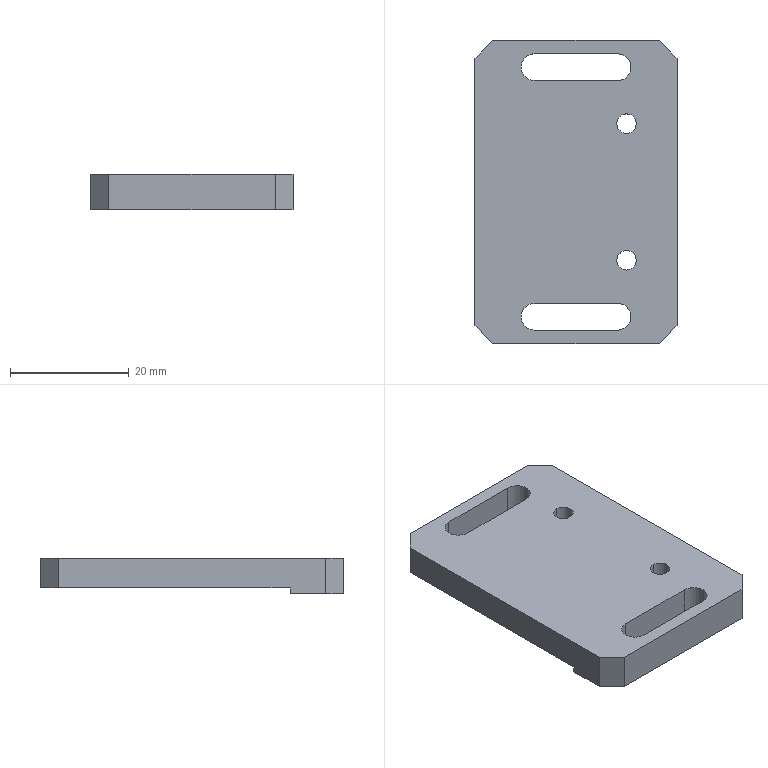Part | STEP file | 11-FG-SZ00711 | 1 solid | 26 faces | box 34 x 51 x 6 mm | volume 7924 mm3 | plane 16 | cylinder 10 | commonest cylinder face diameters 4.5 x6 3.3 x4
STEP:
#1=CARTESIAN_POINT('',(-9.25,21.,6.));
#2=VERTEX_POINT('',#1);
#3=CARTESIAN_POINT('',(-7.,23.25,6.));
#4=VERTEX_POINT('',#3);
#5=CARTESIAN_POINT('',(-7.,21.,6.));
#6=DIRECTION('',(0.,0.,-1.));
#7=DIRECTION('',(1.,0.,0.));
#8=AXIS2_PLACEMENT_3D('',#5,#6,#7);
#9=CIRCLE('',#8,2.25);
#10=EDGE_CURVE('',#2,#4,#9,.T.);
#11=ORIENTED_EDGE('',*,*,#10,.F.);
#12=CARTESIAN_POINT('',(-9.25,21.,1.));
#13=VERTEX_POINT('',#12);
#14=CARTESIAN_POINT('',(-9.25,21.,6.));
#15=DIRECTION('',(0.,0.,-1.));
#16=VECTOR('',#15,1000.);
#17=LINE('',#14,#16);
#18=EDGE_CURVE('',#2,#13,#17,.T.);
#19=ORIENTED_EDGE('',*,*,#18,.T.);
#20=CARTESIAN_POINT('',(-7.,23.25,1.));
#21=VERTEX_POINT('',#20);
#22=CARTESIAN_POINT('',(-7.,21.,1.));
#23=DIRECTION('',(0.,0.,1.));
#24=DIRECTION('',(0.,-1.,0.));
#25=AXIS2_PLACEMENT_3D('',#22,#23,#24);
#26=CIRCLE('',#25,2.25);
#27=EDGE_CURVE('',#21,#13,#26,.T.);
#28=ORIENTED_EDGE('',*,*,#27,.F.);
#29=CARTESIAN_POINT('',(-7.,23.25,6.));
#30=DIRECTION('',(0.,0.,-1.));
#31=VECTOR('',#30,1000.);
#32=LINE('',#29,#31);
#33=EDGE_CURVE('',#4,#21,#32,.T.);
#34=ORIENTED_EDGE('',*,*,#33,.F.);
#35=EDGE_LOOP('',(#11,#19,#28,#34));
#36=FACE_OUTER_BOUND('',#35,.T.);
#37=CARTESIAN_POINT('',(-7.,21.,6.));
#38=DIRECTION('',(0.,0.,-1.));
#39=DIRECTION('',(-1.,0.,0.));
#40=AXIS2_PLACEMENT_3D('',#37,#38,#39);
#41=CYLINDRICAL_SURFACE('',#40,2.25);
#42=ADVANCED_FACE('',(#36),#41,.F.);
#43=CARTESIAN_POINT('',(-9.25,-21.,6.));
#44=VERTEX_POINT('',#43);
#45=CARTESIAN_POINT('',(-7.,-18.75,6.));
#46=VERTEX_POINT('',#45);
#47=CARTESIAN_POINT('',(-7.,-21.,6.));
#48=DIRECTION('',(0.,0.,-1.));
#49=DIRECTION('',(-1.,0.,0.));
#50=AXIS2_PLACEMENT_3D('',#47,#48,#49);
#51=CIRCLE('',#50,2.25);
#52=EDGE_CURVE('',#44,#46,#51,.T.);
#53=ORIENTED_EDGE('',*,*,#52,.F.);
#54=CARTESIAN_POINT('',(-9.25,-21.,0.));
#55=VERTEX_POINT('',#54);
#56=CARTESIAN_POINT('',(-9.25,-21.,6.));
#57=DIRECTION('',(0.,0.,-1.));
#58=VECTOR('',#57,1000.);
#59=LINE('',#56,#58);
#60=EDGE_CURVE('',#44,#55,#59,.T.);
#61=ORIENTED_EDGE('',*,*,#60,.T.);
#62=CARTESIAN_POINT('',(-7.,-18.75,0.));
#63=VERTEX_POINT('',#62);
#64=CARTESIAN_POINT('',(-7.,-21.,0.));
#65=DIRECTION('',(0.,0.,-1.));
#66=DIRECTION('',(-1.,0.,0.));
#67=AXIS2_PLACEMENT_3D('',#64,#65,#66);
#68=CIRCLE('',#67,2.25);
#69=EDGE_CURVE('',#55,#63,#68,.T.);
#70=ORIENTED_EDGE('',*,*,#69,.T.);
#71=CARTESIAN_POINT('',(-7.,-18.75,6.));
#72=DIRECTION('',(0.,0.,-1.));
#73=VECTOR('',#72,1000.);
#74=LINE('',#71,#73);
#75=EDGE_CURVE('',#46,#63,#74,.T.);
#76=ORIENTED_EDGE('',*,*,#75,.F.);
#77=EDGE_LOOP('',(#53,#61,#70,#76));
#78=FACE_OUTER_BOUND('',#77,.T.);
#79=CARTESIAN_POINT('',(-7.,-21.,6.));
#80=DIRECTION('',(0.,0.,-1.));
#81=DIRECTION('',(-1.,0.,0.));
#82=AXIS2_PLACEMENT_3D('',#79,#80,#81);
#83=CYLINDRICAL_SURFACE('',#82,2.25);
#84=ADVANCED_FACE('',(#78),#83,.F.);
#85=CARTESIAN_POINT('',(8.5,-9.85,6.));
#86=VERTEX_POINT('',#85);
#87=CARTESIAN_POINT('',(8.5,-13.15,6.));
#88=VERTEX_POINT('',#87);
#89=CARTESIAN_POINT('',(8.5,-11.5,6.));
#90=DIRECTION('',(0.,0.,1.));
#91=DIRECTION('',(1.,0.,0.));
#92=AXIS2_PLACEMENT_3D('',#89,#90,#91);
#93=CIRCLE('',#92,1.65);
#94=EDGE_CURVE('',#86,#88,#93,.T.);
#95=ORIENTED_EDGE('',*,*,#94,.T.);
#96=CARTESIAN_POINT('',(8.5,-13.15,1.));
#97=VERTEX_POINT('',#96);
#98=CARTESIAN_POINT('',(8.5,-13.15,1.));
#99=DIRECTION('',(0.,0.,-1.));
#100=VECTOR('',#99,1000.);
#101=LINE('',#98,#100);
#102=EDGE_CURVE('',#88,#97,#101,.T.);
#103=ORIENTED_EDGE('',*,*,#102,.T.);
#104=CARTESIAN_POINT('',(8.5,-9.85,1.));
#105=VERTEX_POINT('',#104);
#106=CARTESIAN_POINT('',(8.5,-11.5,1.));
#107=DIRECTION('',(0.,0.,-1.));
#108=DIRECTION('',(0.,1.,0.));
#109=AXIS2_PLACEMENT_3D('',#106,#107,#108);
#110=CIRCLE('',#109,1.65);
#111=EDGE_CURVE('',#97,#105,#110,.T.);
#112=ORIENTED_EDGE('',*,*,#111,.T.);
#113=CARTESIAN_POINT('',(8.5,-9.85,1.));
#114=DIRECTION('',(0.,0.,-1.));
#115=VECTOR('',#114,1000.);
#116=LINE('',#113,#115);
#117=EDGE_CURVE('',#86,#105,#116,.T.);
#118=ORIENTED_EDGE('',*,*,#117,.F.);
#119=EDGE_LOOP('',(#95,#103,#112,#118));
#120=FACE_OUTER_BOUND('',#119,.T.);
#121=CARTESIAN_POINT('',(8.5,-11.5,1.));
#122=DIRECTION('',(0.,0.,-1.));
#123=DIRECTION('',(0.,1.,0.));
#124=AXIS2_PLACEMENT_3D('',#121,#122,#123);
#125=CYLINDRICAL_SURFACE('',#124,1.65);
#126=ADVANCED_FACE('',(#120),#125,.F.);
#127=CARTESIAN_POINT('',(8.5,13.15,6.));
#128=VERTEX_POINT('',#127);
#129=CARTESIAN_POINT('',(8.5,9.85,6.));
#130=VERTEX_POINT('',#129);
#131=CARTESIAN_POINT('',(8.5,11.5,6.));
#132=DIRECTION('',(0.,0.,1.));
#133=DIRECTION('',(1.,0.,0.));
#134=AXIS2_PLACEMENT_3D('',#131,#132,#133);
#135=CIRCLE('',#134,1.65);
#136=EDGE_CURVE('',#128,#130,#135,.T.);
#137=ORIENTED_EDGE('',*,*,#136,.T.);
#138=CARTESIAN_POINT('',(8.5,9.85,1.));
#139=VERTEX_POINT('',#138);
#140=CARTESIAN_POINT('',(8.5,9.85,1.));
#141=DIRECTION('',(0.,0.,-1.));
#142=VECTOR('',#141,1000.);
#143=LINE('',#140,#142);
#144=EDGE_CURVE('',#130,#139,#143,.T.);
#145=ORIENTED_EDGE('',*,*,#144,.T.);
#146=CARTESIAN_POINT('',(8.5,13.15,1.));
#147=VERTEX_POINT('',#146);
#148=CARTESIAN_POINT('',(8.5,11.5,1.));
#149=DIRECTION('',(0.,0.,-1.));
#150=DIRECTION('',(0.,1.,0.));
#151=AXIS2_PLACEMENT_3D('',#148,#149,#150);
#152=CIRCLE('',#151,1.65);
#153=EDGE_CURVE('',#139,#147,#152,.T.);
#154=ORIENTED_EDGE('',*,*,#153,.T.);
#155=CARTESIAN_POINT('',(8.5,13.15,1.));
#156=DIRECTION('',(0.,0.,-1.));
#157=VECTOR('',#156,1000.);
#158=LINE('',#155,#157);
#159=EDGE_CURVE('',#128,#147,#158,.T.);
#160=ORIENTED_EDGE('',*,*,#159,.F.);
#161=EDGE_LOOP('',(#137,#145,#154,#160));
#162=FACE_OUTER_BOUND('',#161,.T.);
#163=CARTESIAN_POINT('',(8.5,11.5,1.));
#164=DIRECTION('',(0.,0.,-1.));
#165=DIRECTION('',(0.,1.,0.));
#166=AXIS2_PLACEMENT_3D('',#163,#164,#165);
#167=CYLINDRICAL_SURFACE('',#166,1.65);
#168=ADVANCED_FACE('',(#162),#167,.F.);
#169=CARTESIAN_POINT('',(17.,22.5,1.));
#170=VERTEX_POINT('',#169);
#171=CARTESIAN_POINT('',(17.,-16.5,1.));
#172=VERTEX_POINT('',#171);
#173=CARTESIAN_POINT('',(17.,25.5,1.));
#174=DIRECTION('',(0.,-1.,0.));
#175=VECTOR('',#174,1000.);
#176=LINE('',#173,#175);
#177=EDGE_CURVE('',#170,#172,#176,.T.);
#178=ORIENTED_EDGE('',*,*,#177,.F.);
#179=CARTESIAN_POINT('',(17.,22.5,6.));
#180=VERTEX_POINT('',#179);
#181=CARTESIAN_POINT('',(17.,22.5,6.));
#182=DIRECTION('',(0.,0.,1.));
#183=VECTOR('',#182,1000.);
#184=LINE('',#181,#183);
#185=EDGE_CURVE('',#170,#180,#184,.T.);
#186=ORIENTED_EDGE('',*,*,#185,.T.);
#187=CARTESIAN_POINT('',(17.,-22.5,6.));
#188=VERTEX_POINT('',#187);
#189=CARTESIAN_POINT('',(17.,25.5,6.));
#190=DIRECTION('',(0.,1.,0.));
#191=VECTOR('',#190,1000.);
#192=LINE('',#189,#191);
#193=EDGE_CURVE('',#188,#180,#192,.T.);
#194=ORIENTED_EDGE('',*,*,#193,.F.);
#195=CARTESIAN_POINT('',(17.,-22.5,0.));
#196=VERTEX_POINT('',#195);
#197=CARTESIAN_POINT('',(17.,-22.5,6.));
#198=DIRECTION('',(0.,0.,-1.));
#199=VECTOR('',#198,1000.);
#200=LINE('',#197,#199);
#201=EDGE_CURVE('',#188,#196,#200,.T.);
#202=ORIENTED_EDGE('',*,*,#201,.T.);
#203=CARTESIAN_POINT('',(17.,-16.5,0.));
#204=VERTEX_POINT('',#203);
#205=CARTESIAN_POINT('',(17.,25.5,0.));
#206=DIRECTION('',(0.,1.,0.));
#207=VECTOR('',#206,1000.);
#208=LINE('',#205,#207);
#209=EDGE_CURVE('',#196,#204,#208,.T.);
#210=ORIENTED_EDGE('',*,*,#209,.T.);
#211=CARTESIAN_POINT('',(17.,-16.5,0.));
#212=DIRECTION('',(0.,0.,-1.));
#213=VECTOR('',#212,1000.);
#214=LINE('',#211,#213);
#215=EDGE_CURVE('',#172,#204,#214,.T.);
#216=ORIENTED_EDGE('',*,*,#215,.F.);
#217=EDGE_LOOP('',(#178,#186,#194,#202,#210,#216));
#218=FACE_OUTER_BOUND('',#217,.T.);
#219=CARTESIAN_POINT('',(17.,25.5,6.));
#220=DIRECTION('',(-1.,0.,0.));
#221=DIRECTION('',(0.,-1.,0.));
#222=AXIS2_PLACEMENT_3D('',#219,#220,#221);
#223=PLANE('',#222);
#224=ADVANCED_FACE('',(#218),#223,.F.);
#225=CARTESIAN_POINT('',(-14.,25.5,1.));
#226=VERTEX_POINT('',#225);
#227=CARTESIAN_POINT('',(14.,25.5,1.));
#228=VERTEX_POINT('',#227);
#229=CARTESIAN_POINT('',(-17.,25.5,1.));
#230=DIRECTION('',(1.,0.,0.));
#231=VECTOR('',#230,1000.);
#232=LINE('',#229,#231);
#233=EDGE_CURVE('',#226,#228,#232,.T.);
#234=ORIENTED_EDGE('',*,*,#233,.F.);
#235=CARTESIAN_POINT('',(-14.,25.5,6.));
#236=VERTEX_POINT('',#235);
#237=CARTESIAN_POINT('',(-14.,25.5,6.));
#238=DIRECTION('',(0.,0.,1.));
#239=VECTOR('',#238,1000.);
#240=LINE('',#237,#239);
#241=EDGE_CURVE('',#226,#236,#240,.T.);
#242=ORIENTED_EDGE('',*,*,#241,.T.);
#243=CARTESIAN_POINT('',(14.,25.5,6.));
#244=VERTEX_POINT('',#243);
#245=CARTESIAN_POINT('',(-17.,25.5,6.));
#246=DIRECTION('',(-1.,0.,0.));
#247=VECTOR('',#246,1000.);
#248=LINE('',#245,#247);
#249=EDGE_CURVE('',#244,#236,#248,.T.);
#250=ORIENTED_EDGE('',*,*,#249,.F.);
#251=CARTESIAN_POINT('',(14.,25.5,6.));
#252=DIRECTION('',(0.,0.,-1.));
#253=VECTOR('',#252,1000.);
#254=LINE('',#251,#253);
#255=EDGE_CURVE('',#244,#228,#254,.T.);
#256=ORIENTED_EDGE('',*,*,#255,.T.);
#257=EDGE_LOOP('',(#234,#242,#250,#256));
#258=FACE_OUTER_BOUND('',#257,.T.);
#259=CARTESIAN_POINT('',(-17.,25.5,6.));
#260=DIRECTION('',(0.,-1.,0.));
#261=DIRECTION('',(0.,0.,-1.));
#262=AXIS2_PLACEMENT_3D('',#259,#260,#261);
#263=PLANE('',#262);
#264=ADVANCED_FACE('',(#258),#263,.F.);
#265=CARTESIAN_POINT('',(-17.,22.5,6.));
#266=VERTEX_POINT('',#265);
#267=CARTESIAN_POINT('',(-17.,-22.5,6.));
#268=VERTEX_POINT('',#267);
#269=CARTESIAN_POINT('',(-17.,25.5,6.));
#270=DIRECTION('',(0.,-1.,0.));
#271=VECTOR('',#270,1000.);
#272=LINE('',#269,#271);
#273=EDGE_CURVE('',#266,#268,#272,.T.);
#274=ORIENTED_EDGE('',*,*,#273,.F.);
#275=CARTESIAN_POINT('',(-17.,22.5,1.));
#276=VERTEX_POINT('',#275);
#277=CARTESIAN_POINT('',(-17.,22.5,6.));
#278=DIRECTION('',(0.,0.,-1.));
#279=VECTOR('',#278,1000.);
#280=LINE('',#277,#279);
#281=EDGE_CURVE('',#266,#276,#280,.T.);
#282=ORIENTED_EDGE('',*,*,#281,.T.);
#283=CARTESIAN_POINT('',(-17.,-16.5,1.));
#284=VERTEX_POINT('',#283);
#285=CARTESIAN_POINT('',(-17.,25.5,1.));
#286=DIRECTION('',(0.,-1.,0.));
#287=VECTOR('',#286,1000.);
#288=LINE('',#285,#287);
#289=EDGE_CURVE('',#276,#284,#288,.T.);
#290=ORIENTED_EDGE('',*,*,#289,.T.);
#291=CARTESIAN_POINT('',(-17.,-16.5,0.));
#292=VERTEX_POINT('',#291);
#293=CARTESIAN_POINT('',(-17.,-16.5,0.));
#294=DIRECTION('',(0.,0.,-1.));
#295=VECTOR('',#294,1000.);
#296=LINE('',#293,#295);
#297=EDGE_CURVE('',#284,#292,#296,.T.);
#298=ORIENTED_EDGE('',*,*,#297,.T.);
#299=CARTESIAN_POINT('',(-17.,-22.5,0.));
#300=VERTEX_POINT('',#299);
#301=CARTESIAN_POINT('',(-17.,25.5,0.));
#302=DIRECTION('',(0.,-1.,0.));
#303=VECTOR('',#302,1000.);
#304=LINE('',#301,#303);
#305=EDGE_CURVE('',#292,#300,#304,.T.);
#306=ORIENTED_EDGE('',*,*,#305,.T.);
#307=CARTESIAN_POINT('',(-17.,-22.5,6.));
#308=DIRECTION('',(0.,0.,1.));
#309=VECTOR('',#308,1000.);
#310=LINE('',#307,#309);
#311=EDGE_CURVE('',#300,#268,#310,.T.);
#312=ORIENTED_EDGE('',*,*,#311,.T.);
#313=EDGE_LOOP('',(#274,#282,#290,#298,#306,#312));
#314=FACE_OUTER_BOUND('',#313,.T.);
#315=CARTESIAN_POINT('',(-17.,25.5,6.));
#316=DIRECTION('',(1.,0.,0.));
#317=DIRECTION('',(0.,1.,0.));
#318=AXIS2_PLACEMENT_3D('',#315,#316,#317);
#319=PLANE('',#318);
#320=ADVANCED_FACE('',(#314),#319,.F.);
#321=CARTESIAN_POINT('',(-14.,-25.5,6.));
#322=VERTEX_POINT('',#321);
#323=CARTESIAN_POINT('',(14.,-25.5,6.));
#324=VERTEX_POINT('',#323);
#325=CARTESIAN_POINT('',(-17.,-25.5,6.));
#326=DIRECTION('',(1.,0.,0.));
#327=VECTOR('',#326,1000.);
#328=LINE('',#325,#327);
#329=EDGE_CURVE('',#322,#324,#328,.T.);
#330=ORIENTED_EDGE('',*,*,#329,.F.);
#331=CARTESIAN_POINT('',(-14.,-25.5,0.));
#332=VERTEX_POINT('',#331);
#333=CARTESIAN_POINT('',(-14.,-25.5,6.));
#334=DIRECTION('',(0.,0.,-1.));
#335=VECTOR('',#334,1000.);
#336=LINE('',#333,#335);
#337=EDGE_CURVE('',#322,#332,#336,.T.);
#338=ORIENTED_EDGE('',*,*,#337,.T.);
#339=CARTESIAN_POINT('',(14.,-25.5,0.));
#340=VERTEX_POINT('',#339);
#341=CARTESIAN_POINT('',(-17.,-25.5,0.));
#342=DIRECTION('',(1.,0.,0.));
#343=VECTOR('',#342,1000.);
#344=LINE('',#341,#343);
#345=EDGE_CURVE('',#332,#340,#344,.T.);
#346=ORIENTED_EDGE('',*,*,#345,.T.);
#347=CARTESIAN_POINT('',(14.,-25.5,6.));
#348=DIRECTION('',(0.,0.,1.));
#349=VECTOR('',#348,1000.);
#350=LINE('',#347,#349);
#351=EDGE_CURVE('',#340,#324,#350,.T.);
#352=ORIENTED_EDGE('',*,*,#351,.T.);
#353=EDGE_LOOP('',(#330,#338,#346,#352));
#354=FACE_OUTER_BOUND('',#353,.T.);
#355=CARTESIAN_POINT('',(-17.,-25.5,6.));
#356=DIRECTION('',(0.,1.,0.));
#357=DIRECTION('',(0.,0.,1.));
#358=AXIS2_PLACEMENT_3D('',#355,#356,#357);
#359=PLANE('',#358);
#360=ADVANCED_FACE('',(#354),#359,.F.);
#361=CARTESIAN_POINT('',(-7.,18.75,6.));
#362=VERTEX_POINT('',#361);
#363=CARTESIAN_POINT('',(-7.,21.,6.));
#364=DIRECTION('',(0.,0.,-1.));
#365=DIRECTION('',(1.,0.,0.));
#366=AXIS2_PLACEMENT_3D('',#363,#364,#365);
#367=CIRCLE('',#366,2.25);
#368=EDGE_CURVE('',#362,#2,#367,.T.);
#369=ORIENTED_EDGE('',*,*,#368,.T.);
#370=ORIENTED_EDGE('',*,*,#10,.T.);
#371=CARTESIAN_POINT('',(7.,23.25,6.));
#372=VERTEX_POINT('',#371);
#373=CARTESIAN_POINT('',(-7.,23.25,6.));
#374=DIRECTION('',(1.,0.,0.));
#375=VECTOR('',#374,1000.);
#376=LINE('',#373,#375);
#377=EDGE_CURVE('',#4,#372,#376,.T.);
#378=ORIENTED_EDGE('',*,*,#377,.T.);
#379=CARTESIAN_POINT('',(7.,18.75,6.));
#380=VERTEX_POINT('',#379);
#381=CARTESIAN_POINT('',(7.,21.,6.));
#382=DIRECTION('',(0.,0.,-1.));
#383=DIRECTION('',(1.,0.,0.));
#384=AXIS2_PLACEMENT_3D('',#381,#382,#383);
#385=CIRCLE('',#384,2.25);
#386=EDGE_CURVE('',#372,#380,#385,.T.);
#387=ORIENTED_EDGE('',*,*,#386,.T.);
#388=CARTESIAN_POINT('',(-7.,18.75,6.));
#389=DIRECTION('',(-1.,0.,0.));
#390=VECTOR('',#389,1000.);
#391=LINE('',#388,#390);
#392=EDGE_CURVE('',#380,#362,#391,.T.);
#393=ORIENTED_EDGE('',*,*,#392,.T.);
#394=EDGE_LOOP('',(#369,#370,#378,#387,#393));
#395=FACE_BOUND('',#394,.T.);
#396=CARTESIAN_POINT('',(-7.,-23.25,6.));
#397=VERTEX_POINT('',#396);
#398=CARTESIAN_POINT('',(-7.,-21.,6.));
#399=DIRECTION('',(0.,0.,-1.));
#400=DIRECTION('',(-1.,0.,0.));
#401=AXIS2_PLACEMENT_3D('',#398,#399,#400);
#402=CIRCLE('',#401,2.25);
#403=EDGE_CURVE('',#397,#44,#402,.T.);
#404=ORIENTED_EDGE('',*,*,#403,.T.);
#405=ORIENTED_EDGE('',*,*,#52,.T.);
#406=CARTESIAN_POINT('',(7.,-18.75,6.));
#407=VERTEX_POINT('',#406);
#408=CARTESIAN_POINT('',(-7.,-18.75,6.));
#409=DIRECTION('',(1.,0.,0.));
#410=VECTOR('',#409,1000.);
#411=LINE('',#408,#410);
#412=EDGE_CURVE('',#46,#407,#411,.T.);
#413=ORIENTED_EDGE('',*,*,#412,.T.);
#414=CARTESIAN_POINT('',(7.,-23.25,6.));
#415=VERTEX_POINT('',#414);
#416=CARTESIAN_POINT('',(7.,-21.,6.));
#417=DIRECTION('',(0.,0.,-1.));
#418=DIRECTION('',(-1.,0.,0.));
#419=AXIS2_PLACEMENT_3D('',#416,#417,#418);
#420=CIRCLE('',#419,2.25);
#421=EDGE_CURVE('',#407,#415,#420,.T.);
#422=ORIENTED_EDGE('',*,*,#421,.T.);
#423=CARTESIAN_POINT('',(-7.,-23.25,6.));
#424=DIRECTION('',(-1.,0.,0.));
#425=VECTOR('',#424,1000.);
#426=LINE('',#423,#425);
#427=EDGE_CURVE('',#415,#397,#426,.T.);
#428=ORIENTED_EDGE('',*,*,#427,.T.);
#429=EDGE_LOOP('',(#404,#405,#413,#422,#428));
#430=FACE_BOUND('',#429,.T.);
#431=ORIENTED_EDGE('',*,*,#94,.F.);
#432=CARTESIAN_POINT('',(8.5,-11.5,6.));
#433=DIRECTION('',(0.,0.,1.));
#434=DIRECTION('',(1.,0.,0.));
#435=AXIS2_PLACEMENT_3D('',#432,#433,#434);
#436=CIRCLE('',#435,1.65);
#437=EDGE_CURVE('',#88,#86,#436,.T.);
#438=ORIENTED_EDGE('',*,*,#437,.F.);
#439=EDGE_LOOP('',(#431,#438));
#440=FACE_BOUND('',#439,.T.);
#441=ORIENTED_EDGE('',*,*,#136,.F.);
#442=CARTESIAN_POINT('',(8.5,11.5,6.));
#443=DIRECTION('',(0.,0.,1.));
#444=DIRECTION('',(1.,0.,0.));
#445=AXIS2_PLACEMENT_3D('',#442,#443,#444);
#446=CIRCLE('',#445,1.65);
#447=EDGE_CURVE('',#130,#128,#446,.T.);
#448=ORIENTED_EDGE('',*,*,#447,.F.);
#449=EDGE_LOOP('',(#441,#448));
#450=FACE_BOUND('',#449,.T.);
#451=ORIENTED_EDGE('',*,*,#249,.T.);
#452=CARTESIAN_POINT('',(-19.75,19.75,6.));
#453=DIRECTION('',(-0.7071,-0.7071,0.));
#454=VECTOR('',#453,1000.);
#455=LINE('',#452,#454);
#456=EDGE_CURVE('',#236,#266,#455,.T.);
#457=ORIENTED_EDGE('',*,*,#456,.T.);
#458=ORIENTED_EDGE('',*,*,#273,.T.);
#459=CARTESIAN_POINT('',(-19.75,-19.75,6.));
#460=DIRECTION('',(0.7071,-0.7071,0.));
#461=VECTOR('',#460,1000.);
#462=LINE('',#459,#461);
#463=EDGE_CURVE('',#268,#322,#462,.T.);
#464=ORIENTED_EDGE('',*,*,#463,.T.);
#465=ORIENTED_EDGE('',*,*,#329,.T.);
#466=CARTESIAN_POINT('',(19.75,-19.75,6.));
#467=DIRECTION('',(0.7071,0.7071,0.));
#468=VECTOR('',#467,1000.);
#469=LINE('',#466,#468);
#470=EDGE_CURVE('',#324,#188,#469,.T.);
#471=ORIENTED_EDGE('',*,*,#470,.T.);
#472=ORIENTED_EDGE('',*,*,#193,.T.);
#473=CARTESIAN_POINT('',(19.75,19.75,6.));
#474=DIRECTION('',(-0.7071,0.7071,0.));
#475=VECTOR('',#474,1000.);
#476=LINE('',#473,#475);
#477=EDGE_CURVE('',#180,#244,#476,.T.);
#478=ORIENTED_EDGE('',*,*,#477,.T.);
#479=EDGE_LOOP('',(#451,#457,#458,#464,#465,#471,#472,#478));
#480=FACE_OUTER_BOUND('',#479,.T.);
#481=CARTESIAN_POINT('',(0.,0.,6.));
#482=DIRECTION('',(0.,0.,1.));
#483=DIRECTION('',(1.,0.,0.));
#484=AXIS2_PLACEMENT_3D('',#481,#482,#483);
#485=PLANE('',#484);
#486=ADVANCED_FACE('',(#395,#430,#440,#450,#480),#485,.T.);
#487=CARTESIAN_POINT('',(7.,-18.75,0.));
#488=VERTEX_POINT('',#487);
#489=CARTESIAN_POINT('',(-7.,-18.75,0.));
#490=DIRECTION('',(1.,0.,0.));
#491=VECTOR('',#490,1000.);
#492=LINE('',#489,#491);
#493=EDGE_CURVE('',#63,#488,#492,.T.);
#494=ORIENTED_EDGE('',*,*,#493,.F.);
#495=ORIENTED_EDGE('',*,*,#69,.F.);
#496=CARTESIAN_POINT('',(-7.,-23.25,0.));
#497=VERTEX_POINT('',#496);
#498=CARTESIAN_POINT('',(-7.,-21.,0.));
#499=DIRECTION('',(0.,0.,-1.));
#500=DIRECTION('',(-1.,0.,0.));
#501=AXIS2_PLACEMENT_3D('',#498,#499,#500);
#502=CIRCLE('',#501,2.25);
#503=EDGE_CURVE('',#497,#55,#502,.T.);
#504=ORIENTED_EDGE('',*,*,#503,.F.);
#505=CARTESIAN_POINT('',(7.,-23.25,0.));
#506=VERTEX_POINT('',#505);
#507=CARTESIAN_POINT('',(-7.,-23.25,0.));
#508=DIRECTION('',(-1.,0.,0.));
#509=VECTOR('',#508,1000.);
#510=LINE('',#507,#509);
#511=EDGE_CURVE('',#506,#497,#510,.T.);
#512=ORIENTED_EDGE('',*,*,#511,.F.);
#513=CARTESIAN_POINT('',(7.,-21.,0.));
#514=DIRECTION('',(0.,0.,-1.));
#515=DIRECTION('',(-1.,0.,0.));
#516=AXIS2_PLACEMENT_3D('',#513,#514,#515);
#517=CIRCLE('',#516,2.25);
#518=EDGE_CURVE('',#488,#506,#517,.T.);
#519=ORIENTED_EDGE('',*,*,#518,.F.);
#520=EDGE_LOOP('',(#494,#495,#504,#512,#519));
#521=FACE_BOUND('',#520,.T.);
#522=ORIENTED_EDGE('',*,*,#345,.F.);
#523=CARTESIAN_POINT('',(-14.,-25.5,0.));
#524=DIRECTION('',(-0.7071,0.7071,0.));
#525=VECTOR('',#524,1000.);
#526=LINE('',#523,#525);
#527=EDGE_CURVE('',#332,#300,#526,.T.);
#528=ORIENTED_EDGE('',*,*,#527,.T.);
#529=ORIENTED_EDGE('',*,*,#305,.F.);
#530=CARTESIAN_POINT('',(-17.,-16.5,0.));
#531=DIRECTION('',(1.,0.,0.));
#532=VECTOR('',#531,1000.);
#533=LINE('',#530,#532);
#534=EDGE_CURVE('',#292,#204,#533,.T.);
#535=ORIENTED_EDGE('',*,*,#534,.T.);
#536=ORIENTED_EDGE('',*,*,#209,.F.);
#537=CARTESIAN_POINT('',(17.,-22.5,0.));
#538=DIRECTION('',(-0.7071,-0.7071,0.));
#539=VECTOR('',#538,1000.);
#540=LINE('',#537,#539);
#541=EDGE_CURVE('',#196,#340,#540,.T.);
#542=ORIENTED_EDGE('',*,*,#541,.T.);
#543=EDGE_LOOP('',(#522,#528,#529,#535,#536,#542));
#544=FACE_OUTER_BOUND('',#543,.T.);
#545=CARTESIAN_POINT('',(0.,0.,0.));
#546=DIRECTION('',(0.,0.,1.));
#547=DIRECTION('',(1.,0.,0.));
#548=AXIS2_PLACEMENT_3D('',#545,#546,#547);
#549=PLANE('',#548);
#550=ADVANCED_FACE('',(#521,#544),#549,.F.);
#551=ORIENTED_EDGE('',*,*,#215,.T.);
#552=ORIENTED_EDGE('',*,*,#534,.F.);
#553=ORIENTED_EDGE('',*,*,#297,.F.);
#554=CARTESIAN_POINT('',(-17.,-16.5,1.));
#555=DIRECTION('',(1.,0.,0.));
#556=VECTOR('',#555,1000.);
#557=LINE('',#554,#556);
#558=EDGE_CURVE('',#284,#172,#557,.T.);
#559=ORIENTED_EDGE('',*,*,#558,.T.);
#560=EDGE_LOOP('',(#551,#552,#553,#559));
#561=FACE_OUTER_BOUND('',#560,.T.);
#562=CARTESIAN_POINT('',(-17.,-16.5,0.));
#563=DIRECTION('',(0.,-1.,0.));
#564=DIRECTION('',(1.,0.,0.));
#565=AXIS2_PLACEMENT_3D('',#562,#563,#564);
#566=PLANE('',#565);
#567=ADVANCED_FACE('',(#561),#566,.F.);
#568=CARTESIAN_POINT('',(7.,23.25,1.));
#569=VERTEX_POINT('',#568);
#570=CARTESIAN_POINT('',(-17.,23.25,1.));
#571=DIRECTION('',(-1.,0.,0.));
#572=VECTOR('',#571,1000.);
#573=LINE('',#570,#572);
#574=EDGE_CURVE('',#569,#21,#573,.T.);
#575=ORIENTED_EDGE('',*,*,#574,.T.);
#576=ORIENTED_EDGE('',*,*,#27,.T.);
#577=CARTESIAN_POINT('',(-7.,18.75,1.));
#578=VERTEX_POINT('',#577);
#579=CARTESIAN_POINT('',(-7.,21.,1.));
#580=DIRECTION('',(0.,0.,1.));
#581=DIRECTION('',(0.,-1.,0.));
#582=AXIS2_PLACEMENT_3D('',#579,#580,#581);
#583=CIRCLE('',#582,2.25);
#584=EDGE_CURVE('',#13,#578,#583,.T.);
#585=ORIENTED_EDGE('',*,*,#584,.T.);
#586=CARTESIAN_POINT('',(7.,18.75,1.));
#587=VERTEX_POINT('',#586);
#588=CARTESIAN_POINT('',(-17.,18.75,1.));
#589=DIRECTION('',(1.,0.,0.));
#590=VECTOR('',#589,1000.);
#591=LINE('',#588,#590);
#592=EDGE_CURVE('',#578,#587,#591,.T.);
#593=ORIENTED_EDGE('',*,*,#592,.T.);
#594=CARTESIAN_POINT('',(7.,21.,1.));
#595=DIRECTION('',(0.,0.,1.));
#596=DIRECTION('',(0.,-1.,0.));
#597=AXIS2_PLACEMENT_3D('',#594,#595,#596);
#598=CIRCLE('',#597,2.25);
#599=EDGE_CURVE('',#587,#569,#598,.T.);
#600=ORIENTED_EDGE('',*,*,#599,.T.);
#601=EDGE_LOOP('',(#575,#576,#585,#593,#600));
#602=FACE_BOUND('',#601,.T.);
#603=CARTESIAN_POINT('',(8.5,-11.5,1.));
#604=DIRECTION('',(0.,0.,-1.));
#605=DIRECTION('',(0.,1.,0.));
#606=AXIS2_PLACEMENT_3D('',#603,#604,#605);
#607=CIRCLE('',#606,1.65);
#608=EDGE_CURVE('',#105,#97,#607,.T.);
#609=ORIENTED_EDGE('',*,*,#608,.F.);
#610=ORIENTED_EDGE('',*,*,#111,.F.);
#611=EDGE_LOOP('',(#609,#610));
#612=FACE_BOUND('',#611,.T.);
#613=CARTESIAN_POINT('',(8.5,11.5,1.));
#614=DIRECTION('',(0.,0.,-1.));
#615=DIRECTION('',(0.,1.,0.));
#616=AXIS2_PLACEMENT_3D('',#613,#614,#615);
#617=CIRCLE('',#616,1.65);
#618=EDGE_CURVE('',#147,#139,#617,.T.);
#619=ORIENTED_EDGE('',*,*,#618,.F.);
#620=ORIENTED_EDGE('',*,*,#153,.F.);
#621=EDGE_LOOP('',(#619,#620));
#622=FACE_BOUND('',#621,.T.);
#623=ORIENTED_EDGE('',*,*,#289,.F.);
#624=CARTESIAN_POINT('',(-17.,22.5,1.));
#625=DIRECTION('',(0.7071,0.7071,0.));
#626=VECTOR('',#625,1000.);
#627=LINE('',#624,#626);
#628=EDGE_CURVE('',#276,#226,#627,.T.);
#629=ORIENTED_EDGE('',*,*,#628,.T.);
#630=ORIENTED_EDGE('',*,*,#233,.T.);
#631=CARTESIAN_POINT('',(14.,25.5,1.));
#632=DIRECTION('',(0.7071,-0.7071,0.));
#633=VECTOR('',#632,1000.);
#634=LINE('',#631,#633);
#635=EDGE_CURVE('',#228,#170,#634,.T.);
#636=ORIENTED_EDGE('',*,*,#635,.T.);
#637=ORIENTED_EDGE('',*,*,#177,.T.);
#638=ORIENTED_EDGE('',*,*,#558,.F.);
#639=EDGE_LOOP('',(#623,#629,#630,#636,#637,#638));
#640=FACE_OUTER_BOUND('',#639,.T.);
#641=CARTESIAN_POINT('',(-17.,25.5,1.));
#642=DIRECTION('',(0.,0.,1.));
#643=DIRECTION('',(0.,-1.,0.));
#644=AXIS2_PLACEMENT_3D('',#641,#642,#643);
#645=PLANE('',#644);
#646=ADVANCED_FACE('',(#602,#612,#622,#640),#645,.F.);
#647=ORIENTED_EDGE('',*,*,#144,.F.);
#648=ORIENTED_EDGE('',*,*,#447,.T.);
#649=ORIENTED_EDGE('',*,*,#159,.T.);
#650=ORIENTED_EDGE('',*,*,#618,.T.);
#651=EDGE_LOOP('',(#647,#648,#649,#650));
#652=FACE_OUTER_BOUND('',#651,.T.);
#653=CARTESIAN_POINT('',(8.5,11.5,1.));
#654=DIRECTION('',(0.,0.,-1.));
#655=DIRECTION('',(0.,1.,0.));
#656=AXIS2_PLACEMENT_3D('',#653,#654,#655);
#657=CYLINDRICAL_SURFACE('',#656,1.65);
#658=ADVANCED_FACE('',(#652),#657,.F.);
#659=ORIENTED_EDGE('',*,*,#102,.F.);
#660=ORIENTED_EDGE('',*,*,#437,.T.);
#661=ORIENTED_EDGE('',*,*,#117,.T.);
#662=ORIENTED_EDGE('',*,*,#608,.T.);
#663=EDGE_LOOP('',(#659,#660,#661,#662));
#664=FACE_OUTER_BOUND('',#663,.T.);
#665=CARTESIAN_POINT('',(8.5,-11.5,1.));
#666=DIRECTION('',(0.,0.,-1.));
#667=DIRECTION('',(0.,1.,0.));
#668=AXIS2_PLACEMENT_3D('',#665,#666,#667);
#669=CYLINDRICAL_SURFACE('',#668,1.65);
#670=ADVANCED_FACE('',(#664),#669,.F.);
#671=ORIENTED_EDGE('',*,*,#60,.F.);
#672=ORIENTED_EDGE('',*,*,#403,.F.);
#673=CARTESIAN_POINT('',(-7.,-23.25,6.));
#674=DIRECTION('',(0.,0.,-1.));
#675=VECTOR('',#674,1000.);
#676=LINE('',#673,#675);
#677=EDGE_CURVE('',#397,#497,#676,.T.);
#678=ORIENTED_EDGE('',*,*,#677,.T.);
#679=ORIENTED_EDGE('',*,*,#503,.T.);
#680=EDGE_LOOP('',(#671,#672,#678,#679));
#681=FACE_OUTER_BOUND('',#680,.T.);
#682=CARTESIAN_POINT('',(-7.,-21.,6.));
#683=DIRECTION('',(0.,0.,-1.));
#684=DIRECTION('',(-1.,0.,0.));
#685=AXIS2_PLACEMENT_3D('',#682,#683,#684);
#686=CYLINDRICAL_SURFACE('',#685,2.25);
#687=ADVANCED_FACE('',(#681),#686,.F.);
#688=ORIENTED_EDGE('',*,*,#511,.T.);
#689=ORIENTED_EDGE('',*,*,#677,.F.);
#690=ORIENTED_EDGE('',*,*,#427,.F.);
#691=CARTESIAN_POINT('',(7.,-23.25,6.));
#692=DIRECTION('',(0.,0.,-1.));
#693=VECTOR('',#692,1000.);
#694=LINE('',#691,#693);
#695=EDGE_CURVE('',#415,#506,#694,.T.);
#696=ORIENTED_EDGE('',*,*,#695,.T.);
#697=EDGE_LOOP('',(#688,#689,#690,#696));
#698=FACE_OUTER_BOUND('',#697,.T.);
#699=CARTESIAN_POINT('',(-7.,-23.25,6.));
#700=DIRECTION('',(0.,-1.,0.));
#701=DIRECTION('',(0.,0.,-1.));
#702=AXIS2_PLACEMENT_3D('',#699,#700,#701);
#703=PLANE('',#702);
#704=ADVANCED_FACE('',(#698),#703,.F.);
#705=ORIENTED_EDGE('',*,*,#518,.T.);
#706=ORIENTED_EDGE('',*,*,#695,.F.);
#707=ORIENTED_EDGE('',*,*,#421,.F.);
#708=CARTESIAN_POINT('',(7.,-18.75,6.));
#709=DIRECTION('',(0.,0.,-1.));
#710=VECTOR('',#709,1000.);
#711=LINE('',#708,#710);
#712=EDGE_CURVE('',#407,#488,#711,.T.);
#713=ORIENTED_EDGE('',*,*,#712,.T.);
#714=EDGE_LOOP('',(#705,#706,#707,#713));
#715=FACE_OUTER_BOUND('',#714,.T.);
#716=CARTESIAN_POINT('',(7.,-21.,6.));
#717=DIRECTION('',(0.,0.,-1.));
#718=DIRECTION('',(-1.,0.,0.));
#719=AXIS2_PLACEMENT_3D('',#716,#717,#718);
#720=CYLINDRICAL_SURFACE('',#719,2.25);
#721=ADVANCED_FACE('',(#715),#720,.F.);
#722=ORIENTED_EDGE('',*,*,#493,.T.);
#723=ORIENTED_EDGE('',*,*,#712,.F.);
#724=ORIENTED_EDGE('',*,*,#412,.F.);
#725=ORIENTED_EDGE('',*,*,#75,.T.);
#726=EDGE_LOOP('',(#722,#723,#724,#725));
#727=FACE_OUTER_BOUND('',#726,.T.);
#728=CARTESIAN_POINT('',(-7.,-18.75,6.));
#729=DIRECTION('',(0.,1.,0.));
#730=DIRECTION('',(-1.,0.,0.));
#731=AXIS2_PLACEMENT_3D('',#728,#729,#730);
#732=PLANE('',#731);
#733=ADVANCED_FACE('',(#727),#732,.F.);
#734=ORIENTED_EDGE('',*,*,#18,.F.);
#735=ORIENTED_EDGE('',*,*,#368,.F.);
#736=CARTESIAN_POINT('',(-7.,18.75,6.));
#737=DIRECTION('',(0.,0.,-1.));
#738=VECTOR('',#737,1000.);
#739=LINE('',#736,#738);
#740=EDGE_CURVE('',#362,#578,#739,.T.);
#741=ORIENTED_EDGE('',*,*,#740,.T.);
#742=ORIENTED_EDGE('',*,*,#584,.F.);
#743=EDGE_LOOP('',(#734,#735,#741,#742));
#744=FACE_OUTER_BOUND('',#743,.T.);
#745=CARTESIAN_POINT('',(-7.,21.,6.));
#746=DIRECTION('',(0.,0.,-1.));
#747=DIRECTION('',(-1.,0.,0.));
#748=AXIS2_PLACEMENT_3D('',#745,#746,#747);
#749=CYLINDRICAL_SURFACE('',#748,2.25);
#750=ADVANCED_FACE('',(#744),#749,.F.);
#751=ORIENTED_EDGE('',*,*,#740,.F.);
#752=ORIENTED_EDGE('',*,*,#392,.F.);
#753=CARTESIAN_POINT('',(7.,18.75,6.));
#754=DIRECTION('',(0.,0.,-1.));
#755=VECTOR('',#754,1000.);
#756=LINE('',#753,#755);
#757=EDGE_CURVE('',#380,#587,#756,.T.);
#758=ORIENTED_EDGE('',*,*,#757,.T.);
#759=ORIENTED_EDGE('',*,*,#592,.F.);
#760=EDGE_LOOP('',(#751,#752,#758,#759));
#761=FACE_OUTER_BOUND('',#760,.T.);
#762=CARTESIAN_POINT('',(-7.,18.75,6.));
#763=DIRECTION('',(0.,-1.,0.));
#764=DIRECTION('',(1.,0.,0.));
#765=AXIS2_PLACEMENT_3D('',#762,#763,#764);
#766=PLANE('',#765);
#767=ADVANCED_FACE('',(#761),#766,.F.);
#768=ORIENTED_EDGE('',*,*,#757,.F.);
#769=ORIENTED_EDGE('',*,*,#386,.F.);
#770=CARTESIAN_POINT('',(7.,23.25,6.));
#771=DIRECTION('',(0.,0.,-1.));
#772=VECTOR('',#771,1000.);
#773=LINE('',#770,#772);
#774=EDGE_CURVE('',#372,#569,#773,.T.);
#775=ORIENTED_EDGE('',*,*,#774,.T.);
#776=ORIENTED_EDGE('',*,*,#599,.F.);
#777=EDGE_LOOP('',(#768,#769,#775,#776));
#778=FACE_OUTER_BOUND('',#777,.T.);
#779=CARTESIAN_POINT('',(7.,21.,6.));
#780=DIRECTION('',(0.,0.,-1.));
#781=DIRECTION('',(-1.,0.,0.));
#782=AXIS2_PLACEMENT_3D('',#779,#780,#781);
#783=CYLINDRICAL_SURFACE('',#782,2.25);
#784=ADVANCED_FACE('',(#778),#783,.F.);
#785=ORIENTED_EDGE('',*,*,#774,.F.);
#786=ORIENTED_EDGE('',*,*,#377,.F.);
#787=ORIENTED_EDGE('',*,*,#33,.T.);
#788=ORIENTED_EDGE('',*,*,#574,.F.);
#789=EDGE_LOOP('',(#785,#786,#787,#788));
#790=FACE_OUTER_BOUND('',#789,.T.);
#791=CARTESIAN_POINT('',(-7.,23.25,6.));
#792=DIRECTION('',(0.,1.,0.));
#793=DIRECTION('',(0.,0.,1.));
#794=AXIS2_PLACEMENT_3D('',#791,#792,#793);
#795=PLANE('',#794);
#796=ADVANCED_FACE('',(#790),#795,.F.);
#797=ORIENTED_EDGE('',*,*,#456,.F.);
#798=ORIENTED_EDGE('',*,*,#241,.F.);
#799=ORIENTED_EDGE('',*,*,#628,.F.);
#800=ORIENTED_EDGE('',*,*,#281,.F.);
#801=EDGE_LOOP('',(#797,#798,#799,#800));
#802=FACE_OUTER_BOUND('',#801,.T.);
#803=CARTESIAN_POINT('',(-17.,22.5,6.));
#804=DIRECTION('',(0.7071,-0.7071,0.));
#805=DIRECTION('',(0.,0.,-1.));
#806=AXIS2_PLACEMENT_3D('',#803,#804,#805);
#807=PLANE('',#806);
#808=ADVANCED_FACE('',(#802),#807,.F.);
#809=ORIENTED_EDGE('',*,*,#477,.F.);
#810=ORIENTED_EDGE('',*,*,#185,.F.);
#811=ORIENTED_EDGE('',*,*,#635,.F.);
#812=ORIENTED_EDGE('',*,*,#255,.F.);
#813=EDGE_LOOP('',(#809,#810,#811,#812));
#814=FACE_OUTER_BOUND('',#813,.T.);
#815=CARTESIAN_POINT('',(14.,25.5,6.));
#816=DIRECTION('',(-0.7071,-0.7071,0.));
#817=DIRECTION('',(0.,0.,-1.));
#818=AXIS2_PLACEMENT_3D('',#815,#816,#817);
#819=PLANE('',#818);
#820=ADVANCED_FACE('',(#814),#819,.F.);
#821=ORIENTED_EDGE('',*,*,#463,.F.);
#822=ORIENTED_EDGE('',*,*,#311,.F.);
#823=ORIENTED_EDGE('',*,*,#527,.F.);
#824=ORIENTED_EDGE('',*,*,#337,.F.);
#825=EDGE_LOOP('',(#821,#822,#823,#824));
#826=FACE_OUTER_BOUND('',#825,.T.);
#827=CARTESIAN_POINT('',(-14.,-25.5,6.));
#828=DIRECTION('',(0.7071,0.7071,0.));
#829=DIRECTION('',(0.,0.,-1.));
#830=AXIS2_PLACEMENT_3D('',#827,#828,#829);
#831=PLANE('',#830);
#832=ADVANCED_FACE('',(#826),#831,.F.);
#833=ORIENTED_EDGE('',*,*,#470,.F.);
#834=ORIENTED_EDGE('',*,*,#351,.F.);
#835=ORIENTED_EDGE('',*,*,#541,.F.);
#836=ORIENTED_EDGE('',*,*,#201,.F.);
#837=EDGE_LOOP('',(#833,#834,#835,#836));
#838=FACE_OUTER_BOUND('',#837,.T.);
#839=CARTESIAN_POINT('',(17.,-22.5,6.));
#840=DIRECTION('',(-0.7071,0.7071,0.));
#841=DIRECTION('',(0.,0.,-1.));
#842=AXIS2_PLACEMENT_3D('',#839,#840,#841);
#843=PLANE('',#842);
#844=ADVANCED_FACE('',(#838),#843,.F.);
#845=CLOSED_SHELL('',(#42,#84,#126,#168,#224,#264,#320,#360,#486,#550,#567,#646,#658,#670,#687,#704,#721,#733,#750,#767,#784,#796,#808,#820,#832,#844));
#846=MANIFOLD_SOLID_BREP('',#845);
#847=CARTESIAN_POINT('',(0.,0.,0.));
#848=DIRECTION('',(0.,0.,1.));
#849=DIRECTION('',(1.,0.,0.));
#850=AXIS2_PLACEMENT_3D('',#847,#848,#849);
#851=(LENGTH_UNIT()NAMED_UNIT(*)SI_UNIT(.MILLI.,.METRE.));
#852=UNCERTAINTY_MEASURE_WITH_UNIT(LENGTH_MEASURE(0.00001),#851,'','');
#853=(NAMED_UNIT(*)PLANE_ANGLE_UNIT()SI_UNIT($,.RADIAN.));
#854=(NAMED_UNIT(*)SI_UNIT($,.STERADIAN.)SOLID_ANGLE_UNIT());
#855=(GEOMETRIC_REPRESENTATION_CONTEXT(3)GLOBAL_UNCERTAINTY_ASSIGNED_CONTEXT((#852))GLOBAL_UNIT_ASSIGNED_CONTEXT((#851,#853,#854))REPRESENTATION_CONTEXT('',''));
#856=ADVANCED_BREP_SHAPE_REPRESENTATION('',(#846,#850),#855);